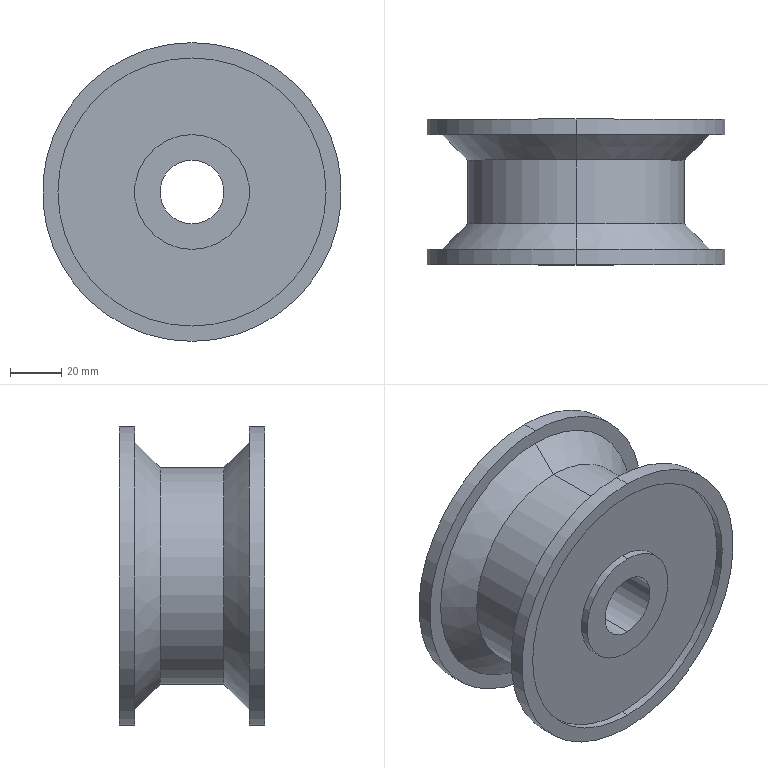Part | SolidWorks | features ICE 2, MirrorPattern 1, Revolution 1 | 1 solid | 28 faces | box 117 x 57 x 117 mm | volume 342775 mm3 | cylinder 16 | plane 8 | cone 4 | commonest cylinder face diameters 45 x4 105 x4 117 x4 25 x2 85 x2
STEP:
#1=CARTESIAN_POINT('',(0.,25.5,-22.5));
#2=VERTEX_POINT('',#1);
#3=CARTESIAN_POINT('',(0.,25.5,22.5));
#4=VERTEX_POINT('',#3);
#5=CARTESIAN_POINT('',(0.,25.5,0.));
#6=DIRECTION('',(0.,-1.,0.));
#7=DIRECTION('',(0.,0.,-1.));
#8=AXIS2_PLACEMENT_3D('',#5,#6,#7);
#9=CIRCLE('',#8,22.5);
#10=EDGE_CURVE('',#2,#4,#9,.T.);
#11=ORIENTED_EDGE('',*,*,#10,.F.);
#12=CARTESIAN_POINT('',(0.,28.5,-22.5));
#13=VERTEX_POINT('',#12);
#14=CARTESIAN_POINT('',(0.,25.5,-22.5));
#15=DIRECTION('',(0.,1.,0.));
#16=VECTOR('',#15,1000.);
#17=LINE('',#14,#16);
#18=EDGE_CURVE('',#2,#13,#17,.T.);
#19=ORIENTED_EDGE('',*,*,#18,.T.);
#20=CARTESIAN_POINT('',(0.,28.5,22.5));
#21=VERTEX_POINT('',#20);
#22=CARTESIAN_POINT('',(0.,28.5,0.));
#23=DIRECTION('',(0.,-1.,0.));
#24=DIRECTION('',(0.,0.,-1.));
#25=AXIS2_PLACEMENT_3D('',#22,#23,#24);
#26=CIRCLE('',#25,22.5);
#27=EDGE_CURVE('',#13,#21,#26,.T.);
#28=ORIENTED_EDGE('',*,*,#27,.T.);
#29=CARTESIAN_POINT('',(0.,25.5,22.5));
#30=DIRECTION('',(0.,1.,0.));
#31=VECTOR('',#30,1000.);
#32=LINE('',#29,#31);
#33=EDGE_CURVE('',#4,#21,#32,.T.);
#34=ORIENTED_EDGE('',*,*,#33,.F.);
#35=EDGE_LOOP('',(#11,#19,#28,#34));
#36=FACE_OUTER_BOUND('',#35,.T.);
#37=CARTESIAN_POINT('',(0.,25.5,0.));
#38=DIRECTION('',(0.,1.,0.));
#39=DIRECTION('',(0.,0.,1.));
#40=AXIS2_PLACEMENT_3D('',#37,#38,#39);
#41=CYLINDRICAL_SURFACE('',#40,22.5);
#42=ADVANCED_FACE('',(#36),#41,.T.);
#43=CARTESIAN_POINT('',(0.,25.5,52.5));
#44=VERTEX_POINT('',#43);
#45=CARTESIAN_POINT('',(0.,25.5,-52.5));
#46=VERTEX_POINT('',#45);
#47=CARTESIAN_POINT('',(0.,25.5,0.));
#48=DIRECTION('',(0.,-1.,0.));
#49=DIRECTION('',(0.,0.,-1.));
#50=AXIS2_PLACEMENT_3D('',#47,#48,#49);
#51=CIRCLE('',#50,52.5);
#52=EDGE_CURVE('',#44,#46,#51,.T.);
#53=ORIENTED_EDGE('',*,*,#52,.T.);
#54=CARTESIAN_POINT('',(0.,28.5,-52.5));
#55=VERTEX_POINT('',#54);
#56=CARTESIAN_POINT('',(0.,25.5,-52.5));
#57=DIRECTION('',(0.,1.,0.));
#58=VECTOR('',#57,1000.);
#59=LINE('',#56,#58);
#60=EDGE_CURVE('',#46,#55,#59,.T.);
#61=ORIENTED_EDGE('',*,*,#60,.T.);
#62=CARTESIAN_POINT('',(0.,28.5,52.5));
#63=VERTEX_POINT('',#62);
#64=CARTESIAN_POINT('',(0.,28.5,0.));
#65=DIRECTION('',(0.,-1.,0.));
#66=DIRECTION('',(0.,0.,-1.));
#67=AXIS2_PLACEMENT_3D('',#64,#65,#66);
#68=CIRCLE('',#67,52.5);
#69=EDGE_CURVE('',#63,#55,#68,.T.);
#70=ORIENTED_EDGE('',*,*,#69,.F.);
#71=CARTESIAN_POINT('',(0.,25.5,52.5));
#72=DIRECTION('',(0.,1.,0.));
#73=VECTOR('',#72,1000.);
#74=LINE('',#71,#73);
#75=EDGE_CURVE('',#44,#63,#74,.T.);
#76=ORIENTED_EDGE('',*,*,#75,.F.);
#77=EDGE_LOOP('',(#53,#61,#70,#76));
#78=FACE_OUTER_BOUND('',#77,.T.);
#79=CARTESIAN_POINT('',(0.,25.5,0.));
#80=DIRECTION('',(0.,1.,0.));
#81=DIRECTION('',(0.,0.,1.));
#82=AXIS2_PLACEMENT_3D('',#79,#80,#81);
#83=CYLINDRICAL_SURFACE('',#82,52.5);
#84=ADVANCED_FACE('',(#78),#83,.F.);
#85=CARTESIAN_POINT('',(0.,-25.5,-22.5));
#86=VERTEX_POINT('',#85);
#87=CARTESIAN_POINT('',(0.,-25.5,22.5));
#88=VERTEX_POINT('',#87);
#89=CARTESIAN_POINT('',(0.,-25.5,0.));
#90=DIRECTION('',(0.,-1.,0.));
#91=DIRECTION('',(0.,0.,-1.));
#92=AXIS2_PLACEMENT_3D('',#89,#90,#91);
#93=CIRCLE('',#92,22.5);
#94=EDGE_CURVE('',#86,#88,#93,.T.);
#95=ORIENTED_EDGE('',*,*,#94,.T.);
#96=CARTESIAN_POINT('',(0.,-28.5,22.5));
#97=VERTEX_POINT('',#96);
#98=CARTESIAN_POINT('',(0.,-25.5,22.5));
#99=DIRECTION('',(0.,-1.,0.));
#100=VECTOR('',#99,1000.);
#101=LINE('',#98,#100);
#102=EDGE_CURVE('',#88,#97,#101,.T.);
#103=ORIENTED_EDGE('',*,*,#102,.T.);
#104=CARTESIAN_POINT('',(0.,-28.5,-22.5));
#105=VERTEX_POINT('',#104);
#106=CARTESIAN_POINT('',(0.,-28.5,0.));
#107=DIRECTION('',(0.,-1.,0.));
#108=DIRECTION('',(0.,0.,-1.));
#109=AXIS2_PLACEMENT_3D('',#106,#107,#108);
#110=CIRCLE('',#109,22.5);
#111=EDGE_CURVE('',#105,#97,#110,.T.);
#112=ORIENTED_EDGE('',*,*,#111,.F.);
#113=CARTESIAN_POINT('',(0.,-25.5,-22.5));
#114=DIRECTION('',(0.,-1.,0.));
#115=VECTOR('',#114,1000.);
#116=LINE('',#113,#115);
#117=EDGE_CURVE('',#86,#105,#116,.T.);
#118=ORIENTED_EDGE('',*,*,#117,.F.);
#119=EDGE_LOOP('',(#95,#103,#112,#118));
#120=FACE_OUTER_BOUND('',#119,.T.);
#121=CARTESIAN_POINT('',(0.,-25.5,0.));
#122=DIRECTION('',(0.,-1.,0.));
#123=DIRECTION('',(0.,0.,-1.));
#124=AXIS2_PLACEMENT_3D('',#121,#122,#123);
#125=CYLINDRICAL_SURFACE('',#124,22.5);
#126=ADVANCED_FACE('',(#120),#125,.T.);
#127=CARTESIAN_POINT('',(0.,-25.5,52.5));
#128=VERTEX_POINT('',#127);
#129=CARTESIAN_POINT('',(0.,-25.5,-52.5));
#130=VERTEX_POINT('',#129);
#131=CARTESIAN_POINT('',(0.,-25.5,0.));
#132=DIRECTION('',(0.,-1.,0.));
#133=DIRECTION('',(0.,0.,-1.));
#134=AXIS2_PLACEMENT_3D('',#131,#132,#133);
#135=CIRCLE('',#134,52.5);
#136=EDGE_CURVE('',#128,#130,#135,.T.);
#137=ORIENTED_EDGE('',*,*,#136,.F.);
#138=CARTESIAN_POINT('',(0.,-28.5,52.5));
#139=VERTEX_POINT('',#138);
#140=CARTESIAN_POINT('',(0.,-25.5,52.5));
#141=DIRECTION('',(0.,-1.,0.));
#142=VECTOR('',#141,1000.);
#143=LINE('',#140,#142);
#144=EDGE_CURVE('',#128,#139,#143,.T.);
#145=ORIENTED_EDGE('',*,*,#144,.T.);
#146=CARTESIAN_POINT('',(0.,-28.5,-52.5));
#147=VERTEX_POINT('',#146);
#148=CARTESIAN_POINT('',(0.,-28.5,0.));
#149=DIRECTION('',(0.,-1.,0.));
#150=DIRECTION('',(0.,0.,-1.));
#151=AXIS2_PLACEMENT_3D('',#148,#149,#150);
#152=CIRCLE('',#151,52.5);
#153=EDGE_CURVE('',#139,#147,#152,.T.);
#154=ORIENTED_EDGE('',*,*,#153,.T.);
#155=CARTESIAN_POINT('',(0.,-25.5,-52.5));
#156=DIRECTION('',(0.,-1.,0.));
#157=VECTOR('',#156,1000.);
#158=LINE('',#155,#157);
#159=EDGE_CURVE('',#130,#147,#158,.T.);
#160=ORIENTED_EDGE('',*,*,#159,.F.);
#161=EDGE_LOOP('',(#137,#145,#154,#160));
#162=FACE_OUTER_BOUND('',#161,.T.);
#163=CARTESIAN_POINT('',(0.,-25.5,0.));
#164=DIRECTION('',(0.,-1.,0.));
#165=DIRECTION('',(0.,0.,-1.));
#166=AXIS2_PLACEMENT_3D('',#163,#164,#165);
#167=CYLINDRICAL_SURFACE('',#166,52.5);
#168=ADVANCED_FACE('',(#162),#167,.F.);
#169=CARTESIAN_POINT('',(0.,28.5,12.5));
#170=VERTEX_POINT('',#169);
#171=CARTESIAN_POINT('',(0.,28.5,-12.5));
#172=VERTEX_POINT('',#171);
#173=CARTESIAN_POINT('',(0.,28.5,0.));
#174=DIRECTION('',(0.,-1.,0.));
#175=DIRECTION('',(0.,0.,-1.));
#176=AXIS2_PLACEMENT_3D('',#173,#174,#175);
#177=CIRCLE('',#176,12.5);
#178=EDGE_CURVE('',#170,#172,#177,.T.);
#179=ORIENTED_EDGE('',*,*,#178,.F.);
#180=CARTESIAN_POINT('',(0.,-28.5,12.5));
#181=VERTEX_POINT('',#180);
#182=CARTESIAN_POINT('',(0.,28.5,12.5));
#183=DIRECTION('',(0.,-1.,0.));
#184=VECTOR('',#183,1000.);
#185=LINE('',#182,#184);
#186=EDGE_CURVE('',#170,#181,#185,.T.);
#187=ORIENTED_EDGE('',*,*,#186,.T.);
#188=CARTESIAN_POINT('',(0.,-28.5,-12.5));
#189=VERTEX_POINT('',#188);
#190=CARTESIAN_POINT('',(0.,-28.5,0.));
#191=DIRECTION('',(0.,-1.,0.));
#192=DIRECTION('',(0.,0.,-1.));
#193=AXIS2_PLACEMENT_3D('',#190,#191,#192);
#194=CIRCLE('',#193,12.5);
#195=EDGE_CURVE('',#181,#189,#194,.T.);
#196=ORIENTED_EDGE('',*,*,#195,.T.);
#197=CARTESIAN_POINT('',(0.,28.5,-12.5));
#198=DIRECTION('',(0.,-1.,0.));
#199=VECTOR('',#198,1000.);
#200=LINE('',#197,#199);
#201=EDGE_CURVE('',#172,#189,#200,.T.);
#202=ORIENTED_EDGE('',*,*,#201,.F.);
#203=EDGE_LOOP('',(#179,#187,#196,#202));
#204=FACE_OUTER_BOUND('',#203,.T.);
#205=CARTESIAN_POINT('',(0.,28.5,0.));
#206=DIRECTION('',(0.,-1.,0.));
#207=DIRECTION('',(0.,0.,-1.));
#208=AXIS2_PLACEMENT_3D('',#205,#206,#207);
#209=CYLINDRICAL_SURFACE('',#208,12.5);
#210=ADVANCED_FACE('',(#204),#209,.F.);
#211=CARTESIAN_POINT('',(0.,-22.5,-58.5));
#212=VERTEX_POINT('',#211);
#213=CARTESIAN_POINT('',(0.,-22.5,58.5));
#214=VERTEX_POINT('',#213);
#215=CARTESIAN_POINT('',(0.,-22.5,0.));
#216=DIRECTION('',(0.,-1.,0.));
#217=DIRECTION('',(0.,0.,-1.));
#218=AXIS2_PLACEMENT_3D('',#215,#216,#217);
#219=CIRCLE('',#218,58.5);
#220=EDGE_CURVE('',#212,#214,#219,.T.);
#221=ORIENTED_EDGE('',*,*,#220,.T.);
#222=CARTESIAN_POINT('',(0.,-28.5,58.5));
#223=VERTEX_POINT('',#222);
#224=CARTESIAN_POINT('',(0.,-28.5,58.5));
#225=DIRECTION('',(0.,-1.,0.));
#226=VECTOR('',#225,1000.);
#227=LINE('',#224,#226);
#228=EDGE_CURVE('',#214,#223,#227,.T.);
#229=ORIENTED_EDGE('',*,*,#228,.T.);
#230=CARTESIAN_POINT('',(0.,-28.5,-58.5));
#231=VERTEX_POINT('',#230);
#232=CARTESIAN_POINT('',(0.,-28.5,0.));
#233=DIRECTION('',(0.,-1.,0.));
#234=DIRECTION('',(0.,0.,-1.));
#235=AXIS2_PLACEMENT_3D('',#232,#233,#234);
#236=CIRCLE('',#235,58.5);
#237=EDGE_CURVE('',#231,#223,#236,.T.);
#238=ORIENTED_EDGE('',*,*,#237,.F.);
#239=CARTESIAN_POINT('',(0.,-28.5,-58.5));
#240=DIRECTION('',(0.,-1.,0.));
#241=VECTOR('',#240,1000.);
#242=LINE('',#239,#241);
#243=EDGE_CURVE('',#212,#231,#242,.T.);
#244=ORIENTED_EDGE('',*,*,#243,.F.);
#245=EDGE_LOOP('',(#221,#229,#238,#244));
#246=FACE_OUTER_BOUND('',#245,.T.);
#247=CARTESIAN_POINT('',(0.,-28.5,0.));
#248=DIRECTION('',(0.,-1.,0.));
#249=DIRECTION('',(0.,0.,-1.));
#250=AXIS2_PLACEMENT_3D('',#247,#248,#249);
#251=CYLINDRICAL_SURFACE('',#250,58.5);
#252=ADVANCED_FACE('',(#246),#251,.T.);
#253=CARTESIAN_POINT('',(0.,-12.5,-42.5));
#254=VERTEX_POINT('',#253);
#255=CARTESIAN_POINT('',(0.,-12.5,42.5));
#256=VERTEX_POINT('',#255);
#257=CARTESIAN_POINT('',(0.,-12.5,0.));
#258=DIRECTION('',(0.,-1.,0.));
#259=DIRECTION('',(0.,0.,-1.));
#260=AXIS2_PLACEMENT_3D('',#257,#258,#259);
#261=CIRCLE('',#260,42.5);
#262=EDGE_CURVE('',#254,#256,#261,.T.);
#263=ORIENTED_EDGE('',*,*,#262,.T.);
#264=CARTESIAN_POINT('',(0.,-22.5,52.5));
#265=VERTEX_POINT('',#264);
#266=CARTESIAN_POINT('',(0.,-22.5,52.5));
#267=DIRECTION('',(0.,-0.7071,0.7071));
#268=VECTOR('',#267,1000.);
#269=LINE('',#266,#268);
#270=EDGE_CURVE('',#256,#265,#269,.T.);
#271=ORIENTED_EDGE('',*,*,#270,.T.);
#272=CARTESIAN_POINT('',(0.,-22.5,-52.5));
#273=VERTEX_POINT('',#272);
#274=CARTESIAN_POINT('',(0.,-22.5,0.));
#275=DIRECTION('',(0.,-1.,0.));
#276=DIRECTION('',(0.,0.,-1.));
#277=AXIS2_PLACEMENT_3D('',#274,#275,#276);
#278=CIRCLE('',#277,52.5);
#279=EDGE_CURVE('',#273,#265,#278,.T.);
#280=ORIENTED_EDGE('',*,*,#279,.F.);
#281=CARTESIAN_POINT('',(0.,-22.5,-52.5));
#282=DIRECTION('',(0.,-0.7071,-0.7071));
#283=VECTOR('',#282,1000.);
#284=LINE('',#281,#283);
#285=EDGE_CURVE('',#254,#273,#284,.T.);
#286=ORIENTED_EDGE('',*,*,#285,.F.);
#287=EDGE_LOOP('',(#263,#271,#280,#286));
#288=FACE_OUTER_BOUND('',#287,.T.);
#289=CARTESIAN_POINT('',(0.,-22.5,0.));
#290=DIRECTION('',(0.,-1.,0.));
#291=DIRECTION('',(0.,0.,-1.));
#292=AXIS2_PLACEMENT_3D('',#289,#290,#291);
#293=CONICAL_SURFACE('',#292,52.5,0.7854);
#294=ADVANCED_FACE('',(#288),#293,.T.);
#295=CARTESIAN_POINT('',(0.,12.5,-42.5));
#296=VERTEX_POINT('',#295);
#297=CARTESIAN_POINT('',(0.,12.5,42.5));
#298=VERTEX_POINT('',#297);
#299=CARTESIAN_POINT('',(0.,12.5,0.));
#300=DIRECTION('',(0.,-1.,0.));
#301=DIRECTION('',(0.,0.,-1.));
#302=AXIS2_PLACEMENT_3D('',#299,#300,#301);
#303=CIRCLE('',#302,42.5);
#304=EDGE_CURVE('',#296,#298,#303,.T.);
#305=ORIENTED_EDGE('',*,*,#304,.T.);
#306=CARTESIAN_POINT('',(0.,-28.5,42.5));
#307=DIRECTION('',(0.,-1.,0.));
#308=VECTOR('',#307,1000.);
#309=LINE('',#306,#308);
#310=EDGE_CURVE('',#298,#256,#309,.T.);
#311=ORIENTED_EDGE('',*,*,#310,.T.);
#312=ORIENTED_EDGE('',*,*,#262,.F.);
#313=CARTESIAN_POINT('',(0.,-28.5,-42.5));
#314=DIRECTION('',(0.,-1.,0.));
#315=VECTOR('',#314,1000.);
#316=LINE('',#313,#315);
#317=EDGE_CURVE('',#296,#254,#316,.T.);
#318=ORIENTED_EDGE('',*,*,#317,.F.);
#319=EDGE_LOOP('',(#305,#311,#312,#318));
#320=FACE_OUTER_BOUND('',#319,.T.);
#321=CARTESIAN_POINT('',(0.,-28.5,0.));
#322=DIRECTION('',(0.,-1.,0.));
#323=DIRECTION('',(0.,0.,-1.));
#324=AXIS2_PLACEMENT_3D('',#321,#322,#323);
#325=CYLINDRICAL_SURFACE('',#324,42.5);
#326=ADVANCED_FACE('',(#320),#325,.T.);
#327=ORIENTED_EDGE('',*,*,#304,.F.);
#328=CARTESIAN_POINT('',(0.,22.5,-52.5));
#329=VERTEX_POINT('',#328);
#330=CARTESIAN_POINT('',(0.,12.5,-42.5));
#331=DIRECTION('',(0.,0.7071,-0.7071));
#332=VECTOR('',#331,1000.);
#333=LINE('',#330,#332);
#334=EDGE_CURVE('',#296,#329,#333,.T.);
#335=ORIENTED_EDGE('',*,*,#334,.T.);
#336=CARTESIAN_POINT('',(0.,22.5,52.5));
#337=VERTEX_POINT('',#336);
#338=CARTESIAN_POINT('',(0.,22.5,0.));
#339=DIRECTION('',(0.,-1.,0.));
#340=DIRECTION('',(0.,0.,-1.));
#341=AXIS2_PLACEMENT_3D('',#338,#339,#340);
#342=CIRCLE('',#341,52.5);
#343=EDGE_CURVE('',#329,#337,#342,.T.);
#344=ORIENTED_EDGE('',*,*,#343,.T.);
#345=CARTESIAN_POINT('',(0.,12.5,42.5));
#346=DIRECTION('',(0.,0.7071,0.7071));
#347=VECTOR('',#346,1000.);
#348=LINE('',#345,#347);
#349=EDGE_CURVE('',#298,#337,#348,.T.);
#350=ORIENTED_EDGE('',*,*,#349,.F.);
#351=EDGE_LOOP('',(#327,#335,#344,#350));
#352=FACE_OUTER_BOUND('',#351,.T.);
#353=CARTESIAN_POINT('',(0.,12.5,0.));
#354=DIRECTION('',(0.,1.,0.));
#355=DIRECTION('',(0.,0.,1.));
#356=AXIS2_PLACEMENT_3D('',#353,#354,#355);
#357=CONICAL_SURFACE('',#356,42.5,0.7854);
#358=ADVANCED_FACE('',(#352),#357,.T.);
#359=CARTESIAN_POINT('',(0.,28.5,-58.5));
#360=VERTEX_POINT('',#359);
#361=CARTESIAN_POINT('',(0.,28.5,58.5));
#362=VERTEX_POINT('',#361);
#363=CARTESIAN_POINT('',(0.,28.5,0.));
#364=DIRECTION('',(0.,-1.,0.));
#365=DIRECTION('',(0.,0.,-1.));
#366=AXIS2_PLACEMENT_3D('',#363,#364,#365);
#367=CIRCLE('',#366,58.5);
#368=EDGE_CURVE('',#360,#362,#367,.T.);
#369=ORIENTED_EDGE('',*,*,#368,.T.);
#370=CARTESIAN_POINT('',(0.,22.5,58.5));
#371=VERTEX_POINT('',#370);
#372=CARTESIAN_POINT('',(0.,-28.5,58.5));
#373=DIRECTION('',(0.,-1.,0.));
#374=VECTOR('',#373,1000.);
#375=LINE('',#372,#374);
#376=EDGE_CURVE('',#362,#371,#375,.T.);
#377=ORIENTED_EDGE('',*,*,#376,.T.);
#378=CARTESIAN_POINT('',(0.,22.5,-58.5));
#379=VERTEX_POINT('',#378);
#380=CARTESIAN_POINT('',(0.,22.5,0.));
#381=DIRECTION('',(0.,-1.,0.));
#382=DIRECTION('',(0.,0.,-1.));
#383=AXIS2_PLACEMENT_3D('',#380,#381,#382);
#384=CIRCLE('',#383,58.5);
#385=EDGE_CURVE('',#379,#371,#384,.T.);
#386=ORIENTED_EDGE('',*,*,#385,.F.);
#387=CARTESIAN_POINT('',(0.,-28.5,-58.5));
#388=DIRECTION('',(0.,-1.,0.));
#389=VECTOR('',#388,1000.);
#390=LINE('',#387,#389);
#391=EDGE_CURVE('',#360,#379,#390,.T.);
#392=ORIENTED_EDGE('',*,*,#391,.F.);
#393=EDGE_LOOP('',(#369,#377,#386,#392));
#394=FACE_OUTER_BOUND('',#393,.T.);
#395=CARTESIAN_POINT('',(0.,-28.5,0.));
#396=DIRECTION('',(0.,-1.,0.));
#397=DIRECTION('',(0.,0.,-1.));
#398=AXIS2_PLACEMENT_3D('',#395,#396,#397);
#399=CYLINDRICAL_SURFACE('',#398,58.5);
#400=ADVANCED_FACE('',(#394),#399,.T.);
#401=ORIENTED_EDGE('',*,*,#368,.F.);
#402=CARTESIAN_POINT('',(0.,28.5,0.));
#403=DIRECTION('',(0.,-1.,0.));
#404=DIRECTION('',(0.,0.,-1.));
#405=AXIS2_PLACEMENT_3D('',#402,#403,#404);
#406=CIRCLE('',#405,58.5);
#407=EDGE_CURVE('',#362,#360,#406,.T.);
#408=ORIENTED_EDGE('',*,*,#407,.F.);
#409=EDGE_LOOP('',(#401,#408));
#410=FACE_OUTER_BOUND('',#409,.T.);
#411=ORIENTED_EDGE('',*,*,#69,.T.);
#412=CARTESIAN_POINT('',(0.,28.5,0.));
#413=DIRECTION('',(0.,-1.,0.));
#414=DIRECTION('',(0.,0.,-1.));
#415=AXIS2_PLACEMENT_3D('',#412,#413,#414);
#416=CIRCLE('',#415,52.5);
#417=EDGE_CURVE('',#55,#63,#416,.T.);
#418=ORIENTED_EDGE('',*,*,#417,.T.);
#419=EDGE_LOOP('',(#411,#418));
#420=FACE_BOUND('',#419,.T.);
#421=CARTESIAN_POINT('',(0.,28.5,0.));
#422=DIRECTION('',(0.,1.,0.));
#423=DIRECTION('',(0.,0.,1.));
#424=AXIS2_PLACEMENT_3D('',#421,#422,#423);
#425=PLANE('',#424);
#426=ADVANCED_FACE('',(#410,#420),#425,.T.);
#427=CARTESIAN_POINT('',(0.,-28.5,0.));
#428=DIRECTION('',(0.,-1.,0.));
#429=DIRECTION('',(0.,0.,-1.));
#430=AXIS2_PLACEMENT_3D('',#427,#428,#429);
#431=CIRCLE('',#430,12.5);
#432=EDGE_CURVE('',#189,#181,#431,.T.);
#433=ORIENTED_EDGE('',*,*,#432,.F.);
#434=ORIENTED_EDGE('',*,*,#195,.F.);
#435=EDGE_LOOP('',(#433,#434));
#436=FACE_BOUND('',#435,.T.);
#437=ORIENTED_EDGE('',*,*,#111,.T.);
#438=CARTESIAN_POINT('',(0.,-28.5,0.));
#439=DIRECTION('',(0.,-1.,0.));
#440=DIRECTION('',(0.,0.,-1.));
#441=AXIS2_PLACEMENT_3D('',#438,#439,#440);
#442=CIRCLE('',#441,22.5);
#443=EDGE_CURVE('',#97,#105,#442,.T.);
#444=ORIENTED_EDGE('',*,*,#443,.T.);
#445=EDGE_LOOP('',(#437,#444));
#446=FACE_OUTER_BOUND('',#445,.T.);
#447=CARTESIAN_POINT('',(0.,-28.5,0.));
#448=DIRECTION('',(0.,-1.,0.));
#449=DIRECTION('',(0.,0.,-1.));
#450=AXIS2_PLACEMENT_3D('',#447,#448,#449);
#451=PLANE('',#450);
#452=ADVANCED_FACE('',(#436,#446),#451,.T.);
#453=CARTESIAN_POINT('',(0.,28.5,0.));
#454=DIRECTION('',(0.,-1.,0.));
#455=DIRECTION('',(0.,0.,-1.));
#456=AXIS2_PLACEMENT_3D('',#453,#454,#455);
#457=CIRCLE('',#456,22.5);
#458=EDGE_CURVE('',#21,#13,#457,.T.);
#459=ORIENTED_EDGE('',*,*,#458,.F.);
#460=ORIENTED_EDGE('',*,*,#27,.F.);
#461=EDGE_LOOP('',(#459,#460));
#462=FACE_OUTER_BOUND('',#461,.T.);
#463=CARTESIAN_POINT('',(0.,28.5,0.));
#464=DIRECTION('',(0.,-1.,0.));
#465=DIRECTION('',(0.,0.,-1.));
#466=AXIS2_PLACEMENT_3D('',#463,#464,#465);
#467=CIRCLE('',#466,12.5);
#468=EDGE_CURVE('',#172,#170,#467,.T.);
#469=ORIENTED_EDGE('',*,*,#468,.T.);
#470=ORIENTED_EDGE('',*,*,#178,.T.);
#471=EDGE_LOOP('',(#469,#470));
#472=FACE_BOUND('',#471,.T.);
#473=CARTESIAN_POINT('',(0.,28.5,0.));
#474=DIRECTION('',(0.,1.,0.));
#475=DIRECTION('',(0.,0.,1.));
#476=AXIS2_PLACEMENT_3D('',#473,#474,#475);
#477=PLANE('',#476);
#478=ADVANCED_FACE('',(#462,#472),#477,.T.);
#479=ORIENTED_EDGE('',*,*,#376,.F.);
#480=ORIENTED_EDGE('',*,*,#407,.T.);
#481=ORIENTED_EDGE('',*,*,#391,.T.);
#482=CARTESIAN_POINT('',(0.,22.5,0.));
#483=DIRECTION('',(0.,-1.,0.));
#484=DIRECTION('',(0.,0.,-1.));
#485=AXIS2_PLACEMENT_3D('',#482,#483,#484);
#486=CIRCLE('',#485,58.5);
#487=EDGE_CURVE('',#371,#379,#486,.T.);
#488=ORIENTED_EDGE('',*,*,#487,.F.);
#489=EDGE_LOOP('',(#479,#480,#481,#488));
#490=FACE_OUTER_BOUND('',#489,.T.);
#491=CARTESIAN_POINT('',(0.,-28.5,0.));
#492=DIRECTION('',(0.,-1.,0.));
#493=DIRECTION('',(0.,0.,-1.));
#494=AXIS2_PLACEMENT_3D('',#491,#492,#493);
#495=CYLINDRICAL_SURFACE('',#494,58.5);
#496=ADVANCED_FACE('',(#490),#495,.T.);
#497=ORIENTED_EDGE('',*,*,#385,.T.);
#498=ORIENTED_EDGE('',*,*,#487,.T.);
#499=EDGE_LOOP('',(#497,#498));
#500=FACE_OUTER_BOUND('',#499,.T.);
#501=CARTESIAN_POINT('',(0.,22.5,0.));
#502=DIRECTION('',(0.,-1.,0.));
#503=DIRECTION('',(0.,0.,-1.));
#504=AXIS2_PLACEMENT_3D('',#501,#502,#503);
#505=CIRCLE('',#504,52.5);
#506=EDGE_CURVE('',#337,#329,#505,.T.);
#507=ORIENTED_EDGE('',*,*,#506,.F.);
#508=ORIENTED_EDGE('',*,*,#343,.F.);
#509=EDGE_LOOP('',(#507,#508));
#510=FACE_BOUND('',#509,.T.);
#511=CARTESIAN_POINT('',(52.5,22.5,0.));
#512=DIRECTION('',(0.,-1.,0.));
#513=DIRECTION('',(0.,0.,-1.));
#514=AXIS2_PLACEMENT_3D('',#511,#512,#513);
#515=PLANE('',#514);
#516=ADVANCED_FACE('',(#500,#510),#515,.T.);
#517=ORIENTED_EDGE('',*,*,#334,.F.);
#518=CARTESIAN_POINT('',(0.,12.5,0.));
#519=DIRECTION('',(0.,-1.,0.));
#520=DIRECTION('',(0.,0.,-1.));
#521=AXIS2_PLACEMENT_3D('',#518,#519,#520);
#522=CIRCLE('',#521,42.5);
#523=EDGE_CURVE('',#298,#296,#522,.T.);
#524=ORIENTED_EDGE('',*,*,#523,.F.);
#525=ORIENTED_EDGE('',*,*,#349,.T.);
#526=ORIENTED_EDGE('',*,*,#506,.T.);
#527=EDGE_LOOP('',(#517,#524,#525,#526));
#528=FACE_OUTER_BOUND('',#527,.T.);
#529=CARTESIAN_POINT('',(0.,12.5,0.));
#530=DIRECTION('',(0.,1.,0.));
#531=DIRECTION('',(0.,0.,1.));
#532=AXIS2_PLACEMENT_3D('',#529,#530,#531);
#533=CONICAL_SURFACE('',#532,42.5,0.7854);
#534=ADVANCED_FACE('',(#528),#533,.T.);
#535=ORIENTED_EDGE('',*,*,#310,.F.);
#536=ORIENTED_EDGE('',*,*,#523,.T.);
#537=ORIENTED_EDGE('',*,*,#317,.T.);
#538=CARTESIAN_POINT('',(0.,-12.5,0.));
#539=DIRECTION('',(0.,-1.,0.));
#540=DIRECTION('',(0.,0.,-1.));
#541=AXIS2_PLACEMENT_3D('',#538,#539,#540);
#542=CIRCLE('',#541,42.5);
#543=EDGE_CURVE('',#256,#254,#542,.T.);
#544=ORIENTED_EDGE('',*,*,#543,.F.);
#545=EDGE_LOOP('',(#535,#536,#537,#544));
#546=FACE_OUTER_BOUND('',#545,.T.);
#547=CARTESIAN_POINT('',(0.,-28.5,0.));
#548=DIRECTION('',(0.,-1.,0.));
#549=DIRECTION('',(0.,0.,-1.));
#550=AXIS2_PLACEMENT_3D('',#547,#548,#549);
#551=CYLINDRICAL_SURFACE('',#550,42.5);
#552=ADVANCED_FACE('',(#546),#551,.T.);
#553=ORIENTED_EDGE('',*,*,#270,.F.);
#554=ORIENTED_EDGE('',*,*,#543,.T.);
#555=ORIENTED_EDGE('',*,*,#285,.T.);
#556=CARTESIAN_POINT('',(0.,-22.5,0.));
#557=DIRECTION('',(0.,-1.,0.));
#558=DIRECTION('',(0.,0.,-1.));
#559=AXIS2_PLACEMENT_3D('',#556,#557,#558);
#560=CIRCLE('',#559,52.5);
#561=EDGE_CURVE('',#265,#273,#560,.T.);
#562=ORIENTED_EDGE('',*,*,#561,.F.);
#563=EDGE_LOOP('',(#553,#554,#555,#562));
#564=FACE_OUTER_BOUND('',#563,.T.);
#565=CARTESIAN_POINT('',(0.,-22.5,0.));
#566=DIRECTION('',(0.,-1.,0.));
#567=DIRECTION('',(0.,0.,-1.));
#568=AXIS2_PLACEMENT_3D('',#565,#566,#567);
#569=CONICAL_SURFACE('',#568,52.5,0.7854);
#570=ADVANCED_FACE('',(#564),#569,.T.);
#571=ORIENTED_EDGE('',*,*,#279,.T.);
#572=ORIENTED_EDGE('',*,*,#561,.T.);
#573=EDGE_LOOP('',(#571,#572));
#574=FACE_BOUND('',#573,.T.);
#575=ORIENTED_EDGE('',*,*,#220,.F.);
#576=CARTESIAN_POINT('',(0.,-22.5,0.));
#577=DIRECTION('',(0.,-1.,0.));
#578=DIRECTION('',(0.,0.,-1.));
#579=AXIS2_PLACEMENT_3D('',#576,#577,#578);
#580=CIRCLE('',#579,58.5);
#581=EDGE_CURVE('',#214,#212,#580,.T.);
#582=ORIENTED_EDGE('',*,*,#581,.F.);
#583=EDGE_LOOP('',(#575,#582));
#584=FACE_OUTER_BOUND('',#583,.T.);
#585=CARTESIAN_POINT('',(52.5,-22.5,0.));
#586=DIRECTION('',(0.,1.,0.));
#587=DIRECTION('',(0.,0.,1.));
#588=AXIS2_PLACEMENT_3D('',#585,#586,#587);
#589=PLANE('',#588);
#590=ADVANCED_FACE('',(#574,#584),#589,.T.);
#591=ORIENTED_EDGE('',*,*,#228,.F.);
#592=ORIENTED_EDGE('',*,*,#581,.T.);
#593=ORIENTED_EDGE('',*,*,#243,.T.);
#594=CARTESIAN_POINT('',(0.,-28.5,0.));
#595=DIRECTION('',(0.,-1.,0.));
#596=DIRECTION('',(0.,0.,-1.));
#597=AXIS2_PLACEMENT_3D('',#594,#595,#596);
#598=CIRCLE('',#597,58.5);
#599=EDGE_CURVE('',#223,#231,#598,.T.);
#600=ORIENTED_EDGE('',*,*,#599,.F.);
#601=EDGE_LOOP('',(#591,#592,#593,#600));
#602=FACE_OUTER_BOUND('',#601,.T.);
#603=CARTESIAN_POINT('',(0.,-28.5,0.));
#604=DIRECTION('',(0.,-1.,0.));
#605=DIRECTION('',(0.,0.,-1.));
#606=AXIS2_PLACEMENT_3D('',#603,#604,#605);
#607=CYLINDRICAL_SURFACE('',#606,58.5);
#608=ADVANCED_FACE('',(#602),#607,.T.);
#609=CARTESIAN_POINT('',(0.,-28.5,0.));
#610=DIRECTION('',(0.,-1.,0.));
#611=DIRECTION('',(0.,0.,-1.));
#612=AXIS2_PLACEMENT_3D('',#609,#610,#611);
#613=CIRCLE('',#612,52.5);
#614=EDGE_CURVE('',#147,#139,#613,.T.);
#615=ORIENTED_EDGE('',*,*,#614,.F.);
#616=ORIENTED_EDGE('',*,*,#153,.F.);
#617=EDGE_LOOP('',(#615,#616));
#618=FACE_BOUND('',#617,.T.);
#619=ORIENTED_EDGE('',*,*,#237,.T.);
#620=ORIENTED_EDGE('',*,*,#599,.T.);
#621=EDGE_LOOP('',(#619,#620));
#622=FACE_OUTER_BOUND('',#621,.T.);
#623=CARTESIAN_POINT('',(0.,-28.5,0.));
#624=DIRECTION('',(0.,-1.,0.));
#625=DIRECTION('',(0.,0.,-1.));
#626=AXIS2_PLACEMENT_3D('',#623,#624,#625);
#627=PLANE('',#626);
#628=ADVANCED_FACE('',(#618,#622),#627,.T.);
#629=ORIENTED_EDGE('',*,*,#186,.F.);
#630=ORIENTED_EDGE('',*,*,#468,.F.);
#631=ORIENTED_EDGE('',*,*,#201,.T.);
#632=ORIENTED_EDGE('',*,*,#432,.T.);
#633=EDGE_LOOP('',(#629,#630,#631,#632));
#634=FACE_OUTER_BOUND('',#633,.T.);
#635=CARTESIAN_POINT('',(0.,28.5,0.));
#636=DIRECTION('',(0.,-1.,0.));
#637=DIRECTION('',(0.,0.,-1.));
#638=AXIS2_PLACEMENT_3D('',#635,#636,#637);
#639=CYLINDRICAL_SURFACE('',#638,12.5);
#640=ADVANCED_FACE('',(#634),#639,.F.);
#641=ORIENTED_EDGE('',*,*,#144,.F.);
#642=CARTESIAN_POINT('',(0.,-25.5,0.));
#643=DIRECTION('',(0.,-1.,0.));
#644=DIRECTION('',(0.,0.,-1.));
#645=AXIS2_PLACEMENT_3D('',#642,#643,#644);
#646=CIRCLE('',#645,52.5);
#647=EDGE_CURVE('',#130,#128,#646,.T.);
#648=ORIENTED_EDGE('',*,*,#647,.F.);
#649=ORIENTED_EDGE('',*,*,#159,.T.);
#650=ORIENTED_EDGE('',*,*,#614,.T.);
#651=EDGE_LOOP('',(#641,#648,#649,#650));
#652=FACE_OUTER_BOUND('',#651,.T.);
#653=CARTESIAN_POINT('',(0.,-25.5,0.));
#654=DIRECTION('',(0.,-1.,0.));
#655=DIRECTION('',(0.,0.,-1.));
#656=AXIS2_PLACEMENT_3D('',#653,#654,#655);
#657=CYLINDRICAL_SURFACE('',#656,52.5);
#658=ADVANCED_FACE('',(#652),#657,.F.);
#659=ORIENTED_EDGE('',*,*,#94,.F.);
#660=CARTESIAN_POINT('',(0.,-25.5,0.));
#661=DIRECTION('',(0.,-1.,0.));
#662=DIRECTION('',(0.,0.,-1.));
#663=AXIS2_PLACEMENT_3D('',#660,#661,#662);
#664=CIRCLE('',#663,22.5);
#665=EDGE_CURVE('',#88,#86,#664,.T.);
#666=ORIENTED_EDGE('',*,*,#665,.F.);
#667=EDGE_LOOP('',(#659,#666));
#668=FACE_BOUND('',#667,.T.);
#669=ORIENTED_EDGE('',*,*,#647,.T.);
#670=ORIENTED_EDGE('',*,*,#136,.T.);
#671=EDGE_LOOP('',(#669,#670));
#672=FACE_OUTER_BOUND('',#671,.T.);
#673=CARTESIAN_POINT('',(0.,-25.5,0.));
#674=DIRECTION('',(0.,-1.,0.));
#675=DIRECTION('',(0.,0.,-1.));
#676=AXIS2_PLACEMENT_3D('',#673,#674,#675);
#677=PLANE('',#676);
#678=ADVANCED_FACE('',(#668,#672),#677,.T.);
#679=ORIENTED_EDGE('',*,*,#102,.F.);
#680=ORIENTED_EDGE('',*,*,#665,.T.);
#681=ORIENTED_EDGE('',*,*,#117,.T.);
#682=ORIENTED_EDGE('',*,*,#443,.F.);
#683=EDGE_LOOP('',(#679,#680,#681,#682));
#684=FACE_OUTER_BOUND('',#683,.T.);
#685=CARTESIAN_POINT('',(0.,-25.5,0.));
#686=DIRECTION('',(0.,-1.,0.));
#687=DIRECTION('',(0.,0.,-1.));
#688=AXIS2_PLACEMENT_3D('',#685,#686,#687);
#689=CYLINDRICAL_SURFACE('',#688,22.5);
#690=ADVANCED_FACE('',(#684),#689,.T.);
#691=ORIENTED_EDGE('',*,*,#52,.F.);
#692=CARTESIAN_POINT('',(0.,25.5,0.));
#693=DIRECTION('',(0.,-1.,0.));
#694=DIRECTION('',(0.,0.,-1.));
#695=AXIS2_PLACEMENT_3D('',#692,#693,#694);
#696=CIRCLE('',#695,52.5);
#697=EDGE_CURVE('',#46,#44,#696,.T.);
#698=ORIENTED_EDGE('',*,*,#697,.F.);
#699=EDGE_LOOP('',(#691,#698));
#700=FACE_OUTER_BOUND('',#699,.T.);
#701=CARTESIAN_POINT('',(0.,25.5,0.));
#702=DIRECTION('',(0.,-1.,0.));
#703=DIRECTION('',(0.,0.,-1.));
#704=AXIS2_PLACEMENT_3D('',#701,#702,#703);
#705=CIRCLE('',#704,22.5);
#706=EDGE_CURVE('',#4,#2,#705,.T.);
#707=ORIENTED_EDGE('',*,*,#706,.T.);
#708=ORIENTED_EDGE('',*,*,#10,.T.);
#709=EDGE_LOOP('',(#707,#708));
#710=FACE_BOUND('',#709,.T.);
#711=CARTESIAN_POINT('',(0.,25.5,0.));
#712=DIRECTION('',(0.,1.,0.));
#713=DIRECTION('',(0.,0.,-1.));
#714=AXIS2_PLACEMENT_3D('',#711,#712,#713);
#715=PLANE('',#714);
#716=ADVANCED_FACE('',(#700,#710),#715,.T.);
#717=ORIENTED_EDGE('',*,*,#60,.F.);
#718=ORIENTED_EDGE('',*,*,#697,.T.);
#719=ORIENTED_EDGE('',*,*,#75,.T.);
#720=ORIENTED_EDGE('',*,*,#417,.F.);
#721=EDGE_LOOP('',(#717,#718,#719,#720));
#722=FACE_OUTER_BOUND('',#721,.T.);
#723=CARTESIAN_POINT('',(0.,25.5,0.));
#724=DIRECTION('',(0.,1.,0.));
#725=DIRECTION('',(0.,0.,1.));
#726=AXIS2_PLACEMENT_3D('',#723,#724,#725);
#727=CYLINDRICAL_SURFACE('',#726,52.5);
#728=ADVANCED_FACE('',(#722),#727,.F.);
#729=ORIENTED_EDGE('',*,*,#18,.F.);
#730=ORIENTED_EDGE('',*,*,#706,.F.);
#731=ORIENTED_EDGE('',*,*,#33,.T.);
#732=ORIENTED_EDGE('',*,*,#458,.T.);
#733=EDGE_LOOP('',(#729,#730,#731,#732));
#734=FACE_OUTER_BOUND('',#733,.T.);
#735=CARTESIAN_POINT('',(0.,25.5,0.));
#736=DIRECTION('',(0.,1.,0.));
#737=DIRECTION('',(0.,0.,1.));
#738=AXIS2_PLACEMENT_3D('',#735,#736,#737);
#739=CYLINDRICAL_SURFACE('',#738,22.5);
#740=ADVANCED_FACE('',(#734),#739,.T.);
#741=CLOSED_SHELL('',(#42,#84,#126,#168,#210,#252,#294,#326,#358,#400,#426,#452,#478,#496,#516,#534,#552,#570,#590,#608,#628,#640,#658,#678,#690,#716,#728,#740));
#742=MANIFOLD_SOLID_BREP('',#741);
#743=CARTESIAN_POINT('',(0.,0.,0.));
#744=DIRECTION('',(0.,0.,1.));
#745=DIRECTION('',(1.,0.,0.));
#746=AXIS2_PLACEMENT_3D('',#743,#744,#745);
#747=(LENGTH_UNIT()NAMED_UNIT(*)SI_UNIT(.MILLI.,.METRE.));
#748=UNCERTAINTY_MEASURE_WITH_UNIT(LENGTH_MEASURE(0.00001),#747,'','');
#749=(NAMED_UNIT(*)PLANE_ANGLE_UNIT()SI_UNIT($,.RADIAN.));
#750=(NAMED_UNIT(*)SI_UNIT($,.STERADIAN.)SOLID_ANGLE_UNIT());
#751=(GEOMETRIC_REPRESENTATION_CONTEXT(3)GLOBAL_UNCERTAINTY_ASSIGNED_CONTEXT((#748))GLOBAL_UNIT_ASSIGNED_CONTEXT((#747,#749,#750))REPRESENTATION_CONTEXT('',''));
#752=ADVANCED_BREP_SHAPE_REPRESENTATION('',(#742,#746),#751);